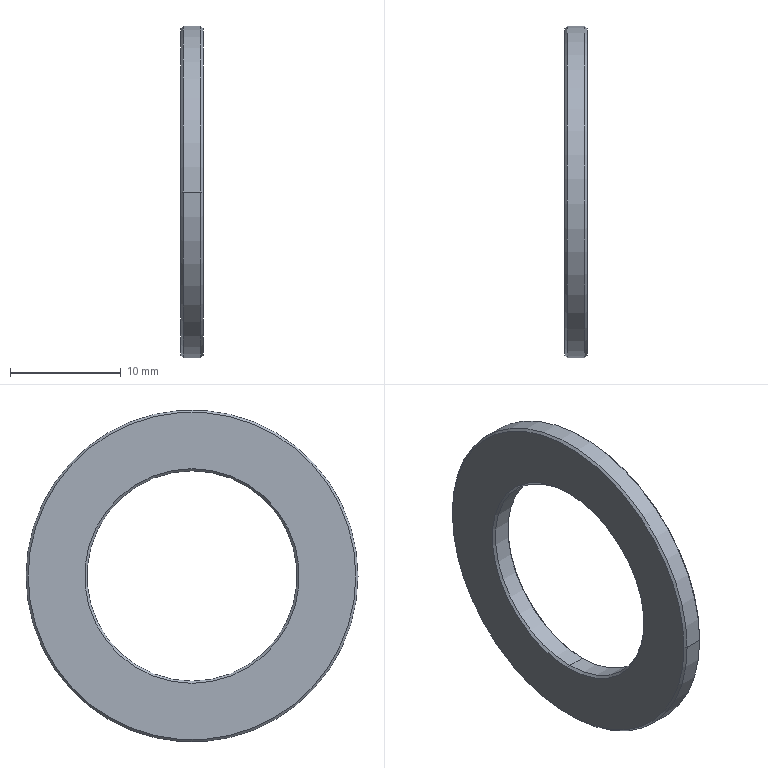Part | STEP file | FWSSS-D30-V19-T2.0 | 1 solid | 14 faces | box 2 x 30 x 30 mm | volume 840.502 mm3 | cone 8 | cylinder 4 | plane 2 | commonest cylinder face diameters 19 x2 30 x2
STEP:
#1=CARTESIAN_POINT('',(0.,0.,0.));
#2=DIRECTION('',(0.,0.,1.));
#3=DIRECTION('',(1.,0.,0.));
#4=AXIS2_PLACEMENT_3D('',#1,#2,#3);
#5=CARTESIAN_POINT('',(0.2,0.,9.5));
#6=VERTEX_POINT('',#5);
#7=CARTESIAN_POINT('',(0.,0.,9.7));
#8=VERTEX_POINT('',#7);
#9=CARTESIAN_POINT('',(0.2,0.,9.5));
#10=DIRECTION('',(-0.7071,0.,0.7071));
#11=VECTOR('',#10,1.);
#12=LINE('',#9,#11);
#13=CARTESIAN_POINT('',(0.2,0.,0.));
#14=DIRECTION('',(-1.,0.,0.));
#15=DIRECTION('',(0.,0.,1.));
#16=AXIS2_PLACEMENT_3D('',#13,#14,#15);
#17=CONICAL_SURFACE('',#16,9.5,0.7854);
#18=CARTESIAN_POINT('',(6.283,0.));
#19=DIRECTION('',(0.,1.));
#20=VECTOR('',#19,1.);
#21=LINE('',#18,#20);
#22=(GEOMETRIC_REPRESENTATION_CONTEXT(2)PARAMETRIC_REPRESENTATION_CONTEXT()REPRESENTATION_CONTEXT('',''));
#23=DEFINITIONAL_REPRESENTATION('',(#21),#22);
#24=PCURVE('',#17,#23);
#25=CARTESIAN_POINT('',(0.2,0.,0.));
#26=DIRECTION('',(-1.,0.,0.));
#27=DIRECTION('',(0.,0.,1.));
#28=AXIS2_PLACEMENT_3D('',#25,#26,#27);
#29=CONICAL_SURFACE('',#28,9.5,0.7854);
#30=CARTESIAN_POINT('',(0.,0.));
#31=DIRECTION('',(0.,1.));
#32=VECTOR('',#31,1.);
#33=LINE('',#30,#32);
#34=(GEOMETRIC_REPRESENTATION_CONTEXT(2)PARAMETRIC_REPRESENTATION_CONTEXT()REPRESENTATION_CONTEXT('',''));
#35=DEFINITIONAL_REPRESENTATION('',(#33),#34);
#36=PCURVE('',#29,#35);
#37=SURFACE_CURVE('',#12,(#24,#36),.PCURVE_S1.);
#38=EDGE_CURVE('',#6,#8,#37,.T.);
#39=ORIENTED_EDGE('',*,*,#38,.T.);
#40=CARTESIAN_POINT('',(0.,0.,-9.7));
#41=VERTEX_POINT('',#40);
#42=CARTESIAN_POINT('',(0.,0.,0.));
#43=DIRECTION('',(1.,0.,0.));
#44=DIRECTION('',(0.,1.,0.));
#45=AXIS2_PLACEMENT_3D('',#42,#43,#44);
#46=CIRCLE('',#45,9.7);
#47=CARTESIAN_POINT('',(7.854,0.2));
#48=DIRECTION('',(-1.,0.));
#49=VECTOR('',#48,1.);
#50=LINE('',#47,#49);
#51=(GEOMETRIC_REPRESENTATION_CONTEXT(2)PARAMETRIC_REPRESENTATION_CONTEXT()REPRESENTATION_CONTEXT('',''));
#52=DEFINITIONAL_REPRESENTATION('',(#50),#51);
#53=PCURVE('',#17,#52);
#54=CARTESIAN_POINT('',(0.,15.,0.));
#55=DIRECTION('',(1.,0.,0.));
#56=DIRECTION('',(0.,1.,0.));
#57=AXIS2_PLACEMENT_3D('',#54,#55,#56);
#58=PLANE('',#57);
#59=CARTESIAN_POINT('',(-15.,0.));
#60=DIRECTION('',(1.,0.));
#61=AXIS2_PLACEMENT_2D('',#59,#60);
#62=CIRCLE('',#61,9.7);
#63=(GEOMETRIC_REPRESENTATION_CONTEXT(2)PARAMETRIC_REPRESENTATION_CONTEXT()REPRESENTATION_CONTEXT('',''));
#64=DEFINITIONAL_REPRESENTATION('',(#62),#63);
#65=PCURVE('',#58,#64);
#66=SURFACE_CURVE('',#46,(#53,#65),.PCURVE_S1.);
#67=EDGE_CURVE('',#8,#41,#66,.T.);
#68=ORIENTED_EDGE('',*,*,#67,.T.);
#69=CARTESIAN_POINT('',(0.2,0.,-9.5));
#70=VERTEX_POINT('',#69);
#71=CARTESIAN_POINT('',(0.2,0.,-9.5));
#72=DIRECTION('',(-0.7071,0.,-0.7071));
#73=VECTOR('',#72,1.);
#74=LINE('',#71,#73);
#75=CARTESIAN_POINT('',(3.142,0.));
#76=DIRECTION('',(0.,1.));
#77=VECTOR('',#76,1.);
#78=LINE('',#75,#77);
#79=(GEOMETRIC_REPRESENTATION_CONTEXT(2)PARAMETRIC_REPRESENTATION_CONTEXT()REPRESENTATION_CONTEXT('',''));
#80=DEFINITIONAL_REPRESENTATION('',(#78),#79);
#81=PCURVE('',#17,#80);
#82=CARTESIAN_POINT('',(3.142,0.));
#83=DIRECTION('',(0.,1.));
#84=VECTOR('',#83,1.);
#85=LINE('',#82,#84);
#86=(GEOMETRIC_REPRESENTATION_CONTEXT(2)PARAMETRIC_REPRESENTATION_CONTEXT()REPRESENTATION_CONTEXT('',''));
#87=DEFINITIONAL_REPRESENTATION('',(#85),#86);
#88=PCURVE('',#29,#87);
#89=SURFACE_CURVE('',#74,(#81,#88),.PCURVE_S1.);
#90=EDGE_CURVE('',#70,#41,#89,.T.);
#91=ORIENTED_EDGE('',*,*,#90,.F.);
#92=CARTESIAN_POINT('',(0.2,0.,0.));
#93=DIRECTION('',(-1.,0.,0.));
#94=DIRECTION('',(0.,0.,-1.));
#95=AXIS2_PLACEMENT_3D('',#92,#93,#94);
#96=CIRCLE('',#95,9.5);
#97=CARTESIAN_POINT('',(3.142,0.));
#98=DIRECTION('',(1.,0.));
#99=VECTOR('',#98,1.);
#100=LINE('',#97,#99);
#101=(GEOMETRIC_REPRESENTATION_CONTEXT(2)PARAMETRIC_REPRESENTATION_CONTEXT()REPRESENTATION_CONTEXT('',''));
#102=DEFINITIONAL_REPRESENTATION('',(#100),#101);
#103=PCURVE('',#17,#102);
#104=CARTESIAN_POINT('',(0.,0.,0.));
#105=DIRECTION('',(1.,0.,0.));
#106=DIRECTION('',(0.,0.,-1.));
#107=AXIS2_PLACEMENT_3D('',#104,#105,#106);
#108=CYLINDRICAL_SURFACE('',#107,9.5);
#109=CARTESIAN_POINT('',(6.283,0.2));
#110=DIRECTION('',(-1.,0.));
#111=VECTOR('',#110,1.);
#112=LINE('',#109,#111);
#113=(GEOMETRIC_REPRESENTATION_CONTEXT(2)PARAMETRIC_REPRESENTATION_CONTEXT()REPRESENTATION_CONTEXT('',''));
#114=DEFINITIONAL_REPRESENTATION('',(#112),#113);
#115=PCURVE('',#108,#114);
#116=SURFACE_CURVE('',#96,(#103,#115),.PCURVE_S1.);
#117=EDGE_CURVE('',#70,#6,#116,.T.);
#118=ORIENTED_EDGE('',*,*,#117,.T.);
#119=EDGE_LOOP('',(#39,#68,#91,#118));
#120=FACE_BOUND('',#119,.F.);
#121=ADVANCED_FACE('',(#120),#17,.F.);
#122=CARTESIAN_POINT('',(1.8,0.,-9.5));
#123=VERTEX_POINT('',#122);
#124=CARTESIAN_POINT('',(2.,0.,-9.7));
#125=VERTEX_POINT('',#124);
#126=CARTESIAN_POINT('',(1.8,0.,-9.5));
#127=DIRECTION('',(0.7071,0.,-0.7071));
#128=VECTOR('',#127,1.);
#129=LINE('',#126,#128);
#130=CARTESIAN_POINT('',(1.8,0.,0.));
#131=DIRECTION('',(1.,0.,0.));
#132=DIRECTION('',(0.,0.,-1.));
#133=AXIS2_PLACEMENT_3D('',#130,#131,#132);
#134=CONICAL_SURFACE('',#133,9.5,0.7854);
#135=CARTESIAN_POINT('',(6.283,0.));
#136=DIRECTION('',(0.,1.));
#137=VECTOR('',#136,1.);
#138=LINE('',#135,#137);
#139=(GEOMETRIC_REPRESENTATION_CONTEXT(2)PARAMETRIC_REPRESENTATION_CONTEXT()REPRESENTATION_CONTEXT('',''));
#140=DEFINITIONAL_REPRESENTATION('',(#138),#139);
#141=PCURVE('',#134,#140);
#142=CARTESIAN_POINT('',(1.8,0.,0.));
#143=DIRECTION('',(1.,0.,0.));
#144=DIRECTION('',(0.,0.,-1.));
#145=AXIS2_PLACEMENT_3D('',#142,#143,#144);
#146=CONICAL_SURFACE('',#145,9.5,0.7854);
#147=CARTESIAN_POINT('',(0.,0.));
#148=DIRECTION('',(0.,1.));
#149=VECTOR('',#148,1.);
#150=LINE('',#147,#149);
#151=(GEOMETRIC_REPRESENTATION_CONTEXT(2)PARAMETRIC_REPRESENTATION_CONTEXT()REPRESENTATION_CONTEXT('',''));
#152=DEFINITIONAL_REPRESENTATION('',(#150),#151);
#153=PCURVE('',#146,#152);
#154=SURFACE_CURVE('',#129,(#141,#153),.PCURVE_S1.);
#155=EDGE_CURVE('',#123,#125,#154,.T.);
#156=ORIENTED_EDGE('',*,*,#155,.T.);
#157=CARTESIAN_POINT('',(2.,0.,9.7));
#158=VERTEX_POINT('',#157);
#159=CARTESIAN_POINT('',(2.,0.,0.));
#160=DIRECTION('',(-1.,0.,0.));
#161=DIRECTION('',(0.,-1.,0.));
#162=AXIS2_PLACEMENT_3D('',#159,#160,#161);
#163=CIRCLE('',#162,9.7);
#164=CARTESIAN_POINT('',(10.996,0.2));
#165=DIRECTION('',(-1.,0.));
#166=VECTOR('',#165,1.);
#167=LINE('',#164,#166);
#168=(GEOMETRIC_REPRESENTATION_CONTEXT(2)PARAMETRIC_REPRESENTATION_CONTEXT()REPRESENTATION_CONTEXT('',''));
#169=DEFINITIONAL_REPRESENTATION('',(#167),#168);
#170=PCURVE('',#134,#169);
#171=CARTESIAN_POINT('',(2.,15.,0.));
#172=DIRECTION('',(-1.,0.,0.));
#173=DIRECTION('',(0.,-1.,0.));
#174=AXIS2_PLACEMENT_3D('',#171,#172,#173);
#175=PLANE('',#174);
#176=CARTESIAN_POINT('',(15.,0.));
#177=DIRECTION('',(1.,0.));
#178=AXIS2_PLACEMENT_2D('',#176,#177);
#179=CIRCLE('',#178,9.7);
#180=(GEOMETRIC_REPRESENTATION_CONTEXT(2)PARAMETRIC_REPRESENTATION_CONTEXT()REPRESENTATION_CONTEXT('',''));
#181=DEFINITIONAL_REPRESENTATION('',(#179),#180);
#182=PCURVE('',#175,#181);
#183=SURFACE_CURVE('',#163,(#170,#182),.PCURVE_S1.);
#184=EDGE_CURVE('',#125,#158,#183,.T.);
#185=ORIENTED_EDGE('',*,*,#184,.T.);
#186=CARTESIAN_POINT('',(1.8,0.,9.5));
#187=VERTEX_POINT('',#186);
#188=CARTESIAN_POINT('',(1.8,0.,9.5));
#189=DIRECTION('',(0.7071,0.,0.7071));
#190=VECTOR('',#189,1.);
#191=LINE('',#188,#190);
#192=CARTESIAN_POINT('',(3.142,0.));
#193=DIRECTION('',(0.,1.));
#194=VECTOR('',#193,1.);
#195=LINE('',#192,#194);
#196=(GEOMETRIC_REPRESENTATION_CONTEXT(2)PARAMETRIC_REPRESENTATION_CONTEXT()REPRESENTATION_CONTEXT('',''));
#197=DEFINITIONAL_REPRESENTATION('',(#195),#196);
#198=PCURVE('',#134,#197);
#199=CARTESIAN_POINT('',(3.142,0.));
#200=DIRECTION('',(0.,1.));
#201=VECTOR('',#200,1.);
#202=LINE('',#199,#201);
#203=(GEOMETRIC_REPRESENTATION_CONTEXT(2)PARAMETRIC_REPRESENTATION_CONTEXT()REPRESENTATION_CONTEXT('',''));
#204=DEFINITIONAL_REPRESENTATION('',(#202),#203);
#205=PCURVE('',#146,#204);
#206=SURFACE_CURVE('',#191,(#198,#205),.PCURVE_S1.);
#207=EDGE_CURVE('',#187,#158,#206,.T.);
#208=ORIENTED_EDGE('',*,*,#207,.F.);
#209=CARTESIAN_POINT('',(1.8,0.,0.));
#210=DIRECTION('',(1.,0.,0.));
#211=DIRECTION('',(0.,0.,1.));
#212=AXIS2_PLACEMENT_3D('',#209,#210,#211);
#213=CIRCLE('',#212,9.5);
#214=CARTESIAN_POINT('',(3.142,0.));
#215=DIRECTION('',(1.,0.));
#216=VECTOR('',#215,1.);
#217=LINE('',#214,#216);
#218=(GEOMETRIC_REPRESENTATION_CONTEXT(2)PARAMETRIC_REPRESENTATION_CONTEXT()REPRESENTATION_CONTEXT('',''));
#219=DEFINITIONAL_REPRESENTATION('',(#217),#218);
#220=PCURVE('',#134,#219);
#221=CARTESIAN_POINT('',(3.142,1.8));
#222=DIRECTION('',(1.,0.));
#223=VECTOR('',#222,1.);
#224=LINE('',#221,#223);
#225=(GEOMETRIC_REPRESENTATION_CONTEXT(2)PARAMETRIC_REPRESENTATION_CONTEXT()REPRESENTATION_CONTEXT('',''));
#226=DEFINITIONAL_REPRESENTATION('',(#224),#225);
#227=PCURVE('',#108,#226);
#228=SURFACE_CURVE('',#213,(#220,#227),.PCURVE_S1.);
#229=EDGE_CURVE('',#187,#123,#228,.T.);
#230=ORIENTED_EDGE('',*,*,#229,.T.);
#231=EDGE_LOOP('',(#156,#185,#208,#230));
#232=FACE_BOUND('',#231,.F.);
#233=ADVANCED_FACE('',(#232),#134,.F.);
#234=CARTESIAN_POINT('',(2.,14.8,0.));
#235=VERTEX_POINT('',#234);
#236=CARTESIAN_POINT('',(2.,-14.8,0.));
#237=VERTEX_POINT('',#236);
#238=CARTESIAN_POINT('',(2.,0.,0.));
#239=DIRECTION('',(1.,0.,0.));
#240=DIRECTION('',(0.,-1.,0.));
#241=AXIS2_PLACEMENT_3D('',#238,#239,#240);
#242=CIRCLE('',#241,14.8);
#243=CARTESIAN_POINT('',(1.8,0.,0.));
#244=DIRECTION('',(-1.,0.,0.));
#245=DIRECTION('',(0.,-1.,0.));
#246=AXIS2_PLACEMENT_3D('',#243,#244,#245);
#247=CONICAL_SURFACE('',#246,15.,0.7854);
#248=CARTESIAN_POINT('',(6.283,-0.2));
#249=DIRECTION('',(-1.,0.));
#250=VECTOR('',#249,1.);
#251=LINE('',#248,#250);
#252=(GEOMETRIC_REPRESENTATION_CONTEXT(2)PARAMETRIC_REPRESENTATION_CONTEXT()REPRESENTATION_CONTEXT('',''));
#253=DEFINITIONAL_REPRESENTATION('',(#251),#252);
#254=PCURVE('',#247,#253);
#255=CARTESIAN_POINT('',(29.8,0.));
#256=CARTESIAN_POINT('',(29.8,-25.634));
#257=CARTESIAN_POINT('',(7.6,-12.817));
#258=CARTESIAN_POINT('',(-14.6,0.));
#259=CARTESIAN_POINT('',(7.6,12.817));
#260=CARTESIAN_POINT('',(29.8,25.634));
#261=CARTESIAN_POINT('',(29.8,0.));
#262=(BOUNDED_CURVE()B_SPLINE_CURVE(2,(#255,#256,#257,#258,#259,#260,#261),.UNSPECIFIED.,.T.,.F.)B_SPLINE_CURVE_WITH_KNOTS((1,2,2,2,2,1),(-2.094,0.,2.094,4.189,6.283,8.378),.UNSPECIFIED.)CURVE()GEOMETRIC_REPRESENTATION_ITEM()RATIONAL_B_SPLINE_CURVE((1.,0.5,1.,0.5,1.,0.5,1.))REPRESENTATION_ITEM(''));
#263=(GEOMETRIC_REPRESENTATION_CONTEXT(2)PARAMETRIC_REPRESENTATION_CONTEXT()REPRESENTATION_CONTEXT('',''));
#264=DEFINITIONAL_REPRESENTATION('',(#262),#263);
#265=PCURVE('',#175,#264);
#266=SURFACE_CURVE('',#242,(#254,#265),.PCURVE_S1.);
#267=EDGE_CURVE('',#235,#237,#266,.T.);
#268=ORIENTED_EDGE('',*,*,#267,.F.);
#269=CARTESIAN_POINT('',(1.8,15.,0.));
#270=VERTEX_POINT('',#269);
#271=CARTESIAN_POINT('',(1.8,15.,0.));
#272=DIRECTION('',(-0.7071,0.7071,0.));
#273=VECTOR('',#272,1.);
#274=LINE('',#271,#273);
#275=CARTESIAN_POINT('',(3.142,0.));
#276=DIRECTION('',(0.,1.));
#277=VECTOR('',#276,1.);
#278=LINE('',#275,#277);
#279=(GEOMETRIC_REPRESENTATION_CONTEXT(2)PARAMETRIC_REPRESENTATION_CONTEXT()REPRESENTATION_CONTEXT('',''));
#280=DEFINITIONAL_REPRESENTATION('',(#278),#279);
#281=PCURVE('',#247,#280);
#282=CARTESIAN_POINT('',(1.8,0.,0.));
#283=DIRECTION('',(-1.,0.,0.));
#284=DIRECTION('',(0.,-1.,0.));
#285=AXIS2_PLACEMENT_3D('',#282,#283,#284);
#286=CONICAL_SURFACE('',#285,15.,0.7854);
#287=CARTESIAN_POINT('',(3.142,0.));
#288=DIRECTION('',(0.,1.));
#289=VECTOR('',#288,1.);
#290=LINE('',#287,#289);
#291=(GEOMETRIC_REPRESENTATION_CONTEXT(2)PARAMETRIC_REPRESENTATION_CONTEXT()REPRESENTATION_CONTEXT('',''));
#292=DEFINITIONAL_REPRESENTATION('',(#290),#291);
#293=PCURVE('',#286,#292);
#294=SURFACE_CURVE('',#274,(#281,#293),.PCURVE_S1.);
#295=EDGE_CURVE('',#235,#270,#294,.T.);
#296=ORIENTED_EDGE('',*,*,#295,.T.);
#297=CARTESIAN_POINT('',(1.8,-15.,0.));
#298=VERTEX_POINT('',#297);
#299=CARTESIAN_POINT('',(1.8,0.,0.));
#300=DIRECTION('',(-1.,0.,0.));
#301=DIRECTION('',(0.,-1.,0.));
#302=AXIS2_PLACEMENT_3D('',#299,#300,#301);
#303=CIRCLE('',#302,15.);
#304=CARTESIAN_POINT('',(0.,0.));
#305=DIRECTION('',(1.,0.));
#306=VECTOR('',#305,1.);
#307=LINE('',#304,#306);
#308=(GEOMETRIC_REPRESENTATION_CONTEXT(2)PARAMETRIC_REPRESENTATION_CONTEXT()REPRESENTATION_CONTEXT('',''));
#309=DEFINITIONAL_REPRESENTATION('',(#307),#308);
#310=PCURVE('',#247,#309);
#311=CARTESIAN_POINT('',(0.,0.,0.));
#312=DIRECTION('',(-1.,0.,0.));
#313=DIRECTION('',(0.,-1.,0.));
#314=AXIS2_PLACEMENT_3D('',#311,#312,#313);
#315=CYLINDRICAL_SURFACE('',#314,15.);
#316=CARTESIAN_POINT('',(0.,-1.8));
#317=DIRECTION('',(1.,0.));
#318=VECTOR('',#317,1.);
#319=LINE('',#316,#318);
#320=(GEOMETRIC_REPRESENTATION_CONTEXT(2)PARAMETRIC_REPRESENTATION_CONTEXT()REPRESENTATION_CONTEXT('',''));
#321=DEFINITIONAL_REPRESENTATION('',(#319),#320);
#322=PCURVE('',#315,#321);
#323=SURFACE_CURVE('',#303,(#310,#322),.PCURVE_S1.);
#324=EDGE_CURVE('',#298,#270,#323,.T.);
#325=ORIENTED_EDGE('',*,*,#324,.F.);
#326=CARTESIAN_POINT('',(1.8,-15.,0.));
#327=DIRECTION('',(-0.7071,-0.7071,0.));
#328=VECTOR('',#327,1.);
#329=LINE('',#326,#328);
#330=CARTESIAN_POINT('',(0.,0.));
#331=DIRECTION('',(0.,1.));
#332=VECTOR('',#331,1.);
#333=LINE('',#330,#332);
#334=(GEOMETRIC_REPRESENTATION_CONTEXT(2)PARAMETRIC_REPRESENTATION_CONTEXT()REPRESENTATION_CONTEXT('',''));
#335=DEFINITIONAL_REPRESENTATION('',(#333),#334);
#336=PCURVE('',#247,#335);
#337=CARTESIAN_POINT('',(6.283,0.));
#338=DIRECTION('',(0.,1.));
#339=VECTOR('',#338,1.);
#340=LINE('',#337,#339);
#341=(GEOMETRIC_REPRESENTATION_CONTEXT(2)PARAMETRIC_REPRESENTATION_CONTEXT()REPRESENTATION_CONTEXT('',''));
#342=DEFINITIONAL_REPRESENTATION('',(#340),#341);
#343=PCURVE('',#286,#342);
#344=SURFACE_CURVE('',#329,(#336,#343),.PCURVE_S1.);
#345=EDGE_CURVE('',#237,#298,#344,.T.);
#346=ORIENTED_EDGE('',*,*,#345,.F.);
#347=EDGE_LOOP('',(#268,#296,#325,#346));
#348=FACE_BOUND('',#347,.T.);
#349=ADVANCED_FACE('',(#348),#247,.T.);
#350=CARTESIAN_POINT('',(0.,-14.8,0.));
#351=VERTEX_POINT('',#350);
#352=CARTESIAN_POINT('',(0.,14.8,0.));
#353=VERTEX_POINT('',#352);
#354=CARTESIAN_POINT('',(0.,0.,0.));
#355=DIRECTION('',(-1.,0.,0.));
#356=DIRECTION('',(0.,1.,0.));
#357=AXIS2_PLACEMENT_3D('',#354,#355,#356);
#358=CIRCLE('',#357,14.8);
#359=CARTESIAN_POINT('',(0.,0.,0.));
#360=DIRECTION('',(1.,0.,0.));
#361=DIRECTION('',(0.,1.,0.));
#362=AXIS2_PLACEMENT_3D('',#359,#360,#361);
#363=CONICAL_SURFACE('',#362,14.8,0.7854);
#364=CARTESIAN_POINT('',(6.283,0.));
#365=DIRECTION('',(-1.,0.));
#366=VECTOR('',#365,1.);
#367=LINE('',#364,#366);
#368=(GEOMETRIC_REPRESENTATION_CONTEXT(2)PARAMETRIC_REPRESENTATION_CONTEXT()REPRESENTATION_CONTEXT('',''));
#369=DEFINITIONAL_REPRESENTATION('',(#367),#368);
#370=PCURVE('',#363,#369);
#371=CARTESIAN_POINT('',(-0.2,0.));
#372=CARTESIAN_POINT('',(-0.2,-25.634));
#373=CARTESIAN_POINT('',(-22.4,-12.817));
#374=CARTESIAN_POINT('',(-44.6,0.));
#375=CARTESIAN_POINT('',(-22.4,12.817));
#376=CARTESIAN_POINT('',(-0.2,25.634));
#377=CARTESIAN_POINT('',(-0.2,0.));
#378=(BOUNDED_CURVE()B_SPLINE_CURVE(2,(#371,#372,#373,#374,#375,#376,#377),.UNSPECIFIED.,.T.,.F.)B_SPLINE_CURVE_WITH_KNOTS((1,2,2,2,2,1),(-2.094,0.,2.094,4.189,6.283,8.378),.UNSPECIFIED.)CURVE()GEOMETRIC_REPRESENTATION_ITEM()RATIONAL_B_SPLINE_CURVE((1.,0.5,1.,0.5,1.,0.5,1.))REPRESENTATION_ITEM(''));
#379=(GEOMETRIC_REPRESENTATION_CONTEXT(2)PARAMETRIC_REPRESENTATION_CONTEXT()REPRESENTATION_CONTEXT('',''));
#380=DEFINITIONAL_REPRESENTATION('',(#378),#379);
#381=PCURVE('',#58,#380);
#382=SURFACE_CURVE('',#358,(#370,#381),.PCURVE_S1.);
#383=EDGE_CURVE('',#351,#353,#382,.T.);
#384=ORIENTED_EDGE('',*,*,#383,.F.);
#385=CARTESIAN_POINT('',(0.2,-15.,0.));
#386=VERTEX_POINT('',#385);
#387=CARTESIAN_POINT('',(0.,-14.8,0.));
#388=DIRECTION('',(0.7071,-0.7071,0.));
#389=VECTOR('',#388,1.);
#390=LINE('',#387,#389);
#391=CARTESIAN_POINT('',(3.142,0.));
#392=DIRECTION('',(0.,1.));
#393=VECTOR('',#392,1.);
#394=LINE('',#391,#393);
#395=(GEOMETRIC_REPRESENTATION_CONTEXT(2)PARAMETRIC_REPRESENTATION_CONTEXT()REPRESENTATION_CONTEXT('',''));
#396=DEFINITIONAL_REPRESENTATION('',(#394),#395);
#397=PCURVE('',#363,#396);
#398=CARTESIAN_POINT('',(0.,0.,0.));
#399=DIRECTION('',(1.,0.,0.));
#400=DIRECTION('',(0.,1.,0.));
#401=AXIS2_PLACEMENT_3D('',#398,#399,#400);
#402=CONICAL_SURFACE('',#401,14.8,0.7854);
#403=CARTESIAN_POINT('',(3.142,0.));
#404=DIRECTION('',(0.,1.));
#405=VECTOR('',#404,1.);
#406=LINE('',#403,#405);
#407=(GEOMETRIC_REPRESENTATION_CONTEXT(2)PARAMETRIC_REPRESENTATION_CONTEXT()REPRESENTATION_CONTEXT('',''));
#408=DEFINITIONAL_REPRESENTATION('',(#406),#407);
#409=PCURVE('',#402,#408);
#410=SURFACE_CURVE('',#390,(#397,#409),.PCURVE_S1.);
#411=EDGE_CURVE('',#351,#386,#410,.T.);
#412=ORIENTED_EDGE('',*,*,#411,.T.);
#413=CARTESIAN_POINT('',(0.2,15.,0.));
#414=VERTEX_POINT('',#413);
#415=CARTESIAN_POINT('',(0.2,0.,0.));
#416=DIRECTION('',(1.,0.,0.));
#417=DIRECTION('',(0.,1.,0.));
#418=AXIS2_PLACEMENT_3D('',#415,#416,#417);
#419=CIRCLE('',#418,15.);
#420=CARTESIAN_POINT('',(0.,0.2));
#421=DIRECTION('',(1.,0.));
#422=VECTOR('',#421,1.);
#423=LINE('',#420,#422);
#424=(GEOMETRIC_REPRESENTATION_CONTEXT(2)PARAMETRIC_REPRESENTATION_CONTEXT()REPRESENTATION_CONTEXT('',''));
#425=DEFINITIONAL_REPRESENTATION('',(#423),#424);
#426=PCURVE('',#363,#425);
#427=CARTESIAN_POINT('',(3.142,-0.2));
#428=DIRECTION('',(-1.,0.));
#429=VECTOR('',#428,1.);
#430=LINE('',#427,#429);
#431=(GEOMETRIC_REPRESENTATION_CONTEXT(2)PARAMETRIC_REPRESENTATION_CONTEXT()REPRESENTATION_CONTEXT('',''));
#432=DEFINITIONAL_REPRESENTATION('',(#430),#431);
#433=PCURVE('',#315,#432);
#434=SURFACE_CURVE('',#419,(#426,#433),.PCURVE_S1.);
#435=EDGE_CURVE('',#414,#386,#434,.T.);
#436=ORIENTED_EDGE('',*,*,#435,.F.);
#437=CARTESIAN_POINT('',(0.,14.8,0.));
#438=DIRECTION('',(0.7071,0.7071,0.));
#439=VECTOR('',#438,1.);
#440=LINE('',#437,#439);
#441=CARTESIAN_POINT('',(0.,0.));
#442=DIRECTION('',(0.,1.));
#443=VECTOR('',#442,1.);
#444=LINE('',#441,#443);
#445=(GEOMETRIC_REPRESENTATION_CONTEXT(2)PARAMETRIC_REPRESENTATION_CONTEXT()REPRESENTATION_CONTEXT('',''));
#446=DEFINITIONAL_REPRESENTATION('',(#444),#445);
#447=PCURVE('',#363,#446);
#448=CARTESIAN_POINT('',(6.283,0.));
#449=DIRECTION('',(0.,1.));
#450=VECTOR('',#449,1.);
#451=LINE('',#448,#450);
#452=(GEOMETRIC_REPRESENTATION_CONTEXT(2)PARAMETRIC_REPRESENTATION_CONTEXT()REPRESENTATION_CONTEXT('',''));
#453=DEFINITIONAL_REPRESENTATION('',(#451),#452);
#454=PCURVE('',#402,#453);
#455=SURFACE_CURVE('',#440,(#447,#454),.PCURVE_S1.);
#456=EDGE_CURVE('',#353,#414,#455,.T.);
#457=ORIENTED_EDGE('',*,*,#456,.F.);
#458=EDGE_LOOP('',(#384,#412,#436,#457));
#459=FACE_BOUND('',#458,.T.);
#460=ADVANCED_FACE('',(#459),#363,.T.);
#461=CARTESIAN_POINT('',(0.,0.,-9.5));
#462=DIRECTION('',(1.,0.,0.));
#463=VECTOR('',#462,1.);
#464=LINE('',#461,#463);
#465=CARTESIAN_POINT('',(6.283,0.));
#466=DIRECTION('',(0.,1.));
#467=VECTOR('',#466,1.);
#468=LINE('',#465,#467);
#469=(GEOMETRIC_REPRESENTATION_CONTEXT(2)PARAMETRIC_REPRESENTATION_CONTEXT()REPRESENTATION_CONTEXT('',''));
#470=DEFINITIONAL_REPRESENTATION('',(#468),#469);
#471=PCURVE('',#108,#470);
#472=CARTESIAN_POINT('',(0.,0.,0.));
#473=DIRECTION('',(1.,0.,0.));
#474=DIRECTION('',(0.,0.,-1.));
#475=AXIS2_PLACEMENT_3D('',#472,#473,#474);
#476=CYLINDRICAL_SURFACE('',#475,9.5);
#477=CARTESIAN_POINT('',(0.,0.));
#478=DIRECTION('',(0.,1.));
#479=VECTOR('',#478,1.);
#480=LINE('',#477,#479);
#481=(GEOMETRIC_REPRESENTATION_CONTEXT(2)PARAMETRIC_REPRESENTATION_CONTEXT()REPRESENTATION_CONTEXT('',''));
#482=DEFINITIONAL_REPRESENTATION('',(#480),#481);
#483=PCURVE('',#476,#482);
#484=SURFACE_CURVE('',#464,(#471,#483),.PCURVE_S1.);
#485=EDGE_CURVE('',#70,#123,#484,.T.);
#486=ORIENTED_EDGE('',*,*,#485,.T.);
#487=ORIENTED_EDGE('',*,*,#229,.F.);
#488=CARTESIAN_POINT('',(0.,0.,9.5));
#489=DIRECTION('',(1.,0.,0.));
#490=VECTOR('',#489,1.);
#491=LINE('',#488,#490);
#492=CARTESIAN_POINT('',(3.142,0.));
#493=DIRECTION('',(0.,1.));
#494=VECTOR('',#493,1.);
#495=LINE('',#492,#494);
#496=(GEOMETRIC_REPRESENTATION_CONTEXT(2)PARAMETRIC_REPRESENTATION_CONTEXT()REPRESENTATION_CONTEXT('',''));
#497=DEFINITIONAL_REPRESENTATION('',(#495),#496);
#498=PCURVE('',#108,#497);
#499=CARTESIAN_POINT('',(3.142,0.));
#500=DIRECTION('',(0.,1.));
#501=VECTOR('',#500,1.);
#502=LINE('',#499,#501);
#503=(GEOMETRIC_REPRESENTATION_CONTEXT(2)PARAMETRIC_REPRESENTATION_CONTEXT()REPRESENTATION_CONTEXT('',''));
#504=DEFINITIONAL_REPRESENTATION('',(#502),#503);
#505=PCURVE('',#476,#504);
#506=SURFACE_CURVE('',#491,(#498,#505),.PCURVE_S1.);
#507=EDGE_CURVE('',#6,#187,#506,.T.);
#508=ORIENTED_EDGE('',*,*,#507,.F.);
#509=ORIENTED_EDGE('',*,*,#117,.F.);
#510=EDGE_LOOP('',(#486,#487,#508,#509));
#511=FACE_BOUND('',#510,.F.);
#512=ADVANCED_FACE('',(#511),#108,.F.);
#513=ORIENTED_EDGE('',*,*,#324,.T.);
#514=CARTESIAN_POINT('',(0.,15.,0.));
#515=DIRECTION('',(-1.,0.,0.));
#516=VECTOR('',#515,1.);
#517=LINE('',#514,#516);
#518=CARTESIAN_POINT('',(3.142,0.));
#519=DIRECTION('',(0.,1.));
#520=VECTOR('',#519,1.);
#521=LINE('',#518,#520);
#522=(GEOMETRIC_REPRESENTATION_CONTEXT(2)PARAMETRIC_REPRESENTATION_CONTEXT()REPRESENTATION_CONTEXT('',''));
#523=DEFINITIONAL_REPRESENTATION('',(#521),#522);
#524=PCURVE('',#315,#523);
#525=CARTESIAN_POINT('',(0.,0.,0.));
#526=DIRECTION('',(-1.,0.,0.));
#527=DIRECTION('',(0.,-1.,0.));
#528=AXIS2_PLACEMENT_3D('',#525,#526,#527);
#529=CYLINDRICAL_SURFACE('',#528,15.);
#530=CARTESIAN_POINT('',(3.142,0.));
#531=DIRECTION('',(0.,1.));
#532=VECTOR('',#531,1.);
#533=LINE('',#530,#532);
#534=(GEOMETRIC_REPRESENTATION_CONTEXT(2)PARAMETRIC_REPRESENTATION_CONTEXT()REPRESENTATION_CONTEXT('',''));
#535=DEFINITIONAL_REPRESENTATION('',(#533),#534);
#536=PCURVE('',#529,#535);
#537=SURFACE_CURVE('',#517,(#524,#536),.PCURVE_S1.);
#538=EDGE_CURVE('',#270,#414,#537,.T.);
#539=ORIENTED_EDGE('',*,*,#538,.T.);
#540=ORIENTED_EDGE('',*,*,#435,.T.);
#541=CARTESIAN_POINT('',(0.,-15.,0.));
#542=DIRECTION('',(-1.,0.,0.));
#543=VECTOR('',#542,1.);
#544=LINE('',#541,#543);
#545=CARTESIAN_POINT('',(0.,0.));
#546=DIRECTION('',(0.,1.));
#547=VECTOR('',#546,1.);
#548=LINE('',#545,#547);
#549=(GEOMETRIC_REPRESENTATION_CONTEXT(2)PARAMETRIC_REPRESENTATION_CONTEXT()REPRESENTATION_CONTEXT('',''));
#550=DEFINITIONAL_REPRESENTATION('',(#548),#549);
#551=PCURVE('',#315,#550);
#552=CARTESIAN_POINT('',(6.283,0.));
#553=DIRECTION('',(0.,1.));
#554=VECTOR('',#553,1.);
#555=LINE('',#552,#554);
#556=(GEOMETRIC_REPRESENTATION_CONTEXT(2)PARAMETRIC_REPRESENTATION_CONTEXT()REPRESENTATION_CONTEXT('',''));
#557=DEFINITIONAL_REPRESENTATION('',(#555),#556);
#558=PCURVE('',#529,#557);
#559=SURFACE_CURVE('',#544,(#551,#558),.PCURVE_S1.);
#560=EDGE_CURVE('',#298,#386,#559,.T.);
#561=ORIENTED_EDGE('',*,*,#560,.F.);
#562=EDGE_LOOP('',(#513,#539,#540,#561));
#563=FACE_BOUND('',#562,.T.);
#564=ADVANCED_FACE('',(#563),#315,.T.);
#565=ORIENTED_EDGE('',*,*,#184,.T.);
#566=CARTESIAN_POINT('',(2.,0.,0.));
#567=DIRECTION('',(-1.,0.,0.));
#568=DIRECTION('',(0.,-1.,0.));
#569=AXIS2_PLACEMENT_3D('',#566,#567,#568);
#570=CIRCLE('',#569,9.7);
#571=CARTESIAN_POINT('',(15.,0.));
#572=DIRECTION('',(1.,0.));
#573=AXIS2_PLACEMENT_2D('',#571,#572);
#574=CIRCLE('',#573,9.7);
#575=(GEOMETRIC_REPRESENTATION_CONTEXT(2)PARAMETRIC_REPRESENTATION_CONTEXT()REPRESENTATION_CONTEXT('',''));
#576=DEFINITIONAL_REPRESENTATION('',(#574),#575);
#577=PCURVE('',#175,#576);
#578=CARTESIAN_POINT('',(4.712,0.2));
#579=DIRECTION('',(-1.,0.));
#580=VECTOR('',#579,1.);
#581=LINE('',#578,#580);
#582=(GEOMETRIC_REPRESENTATION_CONTEXT(2)PARAMETRIC_REPRESENTATION_CONTEXT()REPRESENTATION_CONTEXT('',''));
#583=DEFINITIONAL_REPRESENTATION('',(#581),#582);
#584=PCURVE('',#146,#583);
#585=SURFACE_CURVE('',#570,(#577,#584),.PCURVE_S1.);
#586=EDGE_CURVE('',#158,#125,#585,.T.);
#587=ORIENTED_EDGE('',*,*,#586,.T.);
#588=EDGE_LOOP('',(#565,#587));
#589=FACE_BOUND('',#588,.T.);
#590=CARTESIAN_POINT('',(2.,0.,0.));
#591=DIRECTION('',(1.,0.,0.));
#592=DIRECTION('',(0.,-1.,0.));
#593=AXIS2_PLACEMENT_3D('',#590,#591,#592);
#594=CIRCLE('',#593,14.8);
#595=CARTESIAN_POINT('',(29.8,0.));
#596=CARTESIAN_POINT('',(29.8,-25.634));
#597=CARTESIAN_POINT('',(7.6,-12.817));
#598=CARTESIAN_POINT('',(-14.6,0.));
#599=CARTESIAN_POINT('',(7.6,12.817));
#600=CARTESIAN_POINT('',(29.8,25.634));
#601=CARTESIAN_POINT('',(29.8,0.));
#602=(BOUNDED_CURVE()B_SPLINE_CURVE(2,(#595,#596,#597,#598,#599,#600,#601),.UNSPECIFIED.,.T.,.F.)B_SPLINE_CURVE_WITH_KNOTS((1,2,2,2,2,1),(-2.094,0.,2.094,4.189,6.283,8.378),.UNSPECIFIED.)CURVE()GEOMETRIC_REPRESENTATION_ITEM()RATIONAL_B_SPLINE_CURVE((1.,0.5,1.,0.5,1.,0.5,1.))REPRESENTATION_ITEM(''));
#603=(GEOMETRIC_REPRESENTATION_CONTEXT(2)PARAMETRIC_REPRESENTATION_CONTEXT()REPRESENTATION_CONTEXT('',''));
#604=DEFINITIONAL_REPRESENTATION('',(#602),#603);
#605=PCURVE('',#175,#604);
#606=CARTESIAN_POINT('',(6.283,-0.2));
#607=DIRECTION('',(-1.,0.));
#608=VECTOR('',#607,1.);
#609=LINE('',#606,#608);
#610=(GEOMETRIC_REPRESENTATION_CONTEXT(2)PARAMETRIC_REPRESENTATION_CONTEXT()REPRESENTATION_CONTEXT('',''));
#611=DEFINITIONAL_REPRESENTATION('',(#609),#610);
#612=PCURVE('',#286,#611);
#613=SURFACE_CURVE('',#594,(#605,#612),.PCURVE_S1.);
#614=EDGE_CURVE('',#237,#235,#613,.T.);
#615=ORIENTED_EDGE('',*,*,#614,.T.);
#616=ORIENTED_EDGE('',*,*,#267,.T.);
#617=EDGE_LOOP('',(#615,#616));
#618=FACE_BOUND('',#617,.T.);
#619=ADVANCED_FACE('',(#589,#618),#175,.F.);
#620=ORIENTED_EDGE('',*,*,#67,.T.);
#621=CARTESIAN_POINT('',(0.,0.,0.));
#622=DIRECTION('',(1.,0.,0.));
#623=DIRECTION('',(0.,1.,0.));
#624=AXIS2_PLACEMENT_3D('',#621,#622,#623);
#625=CIRCLE('',#624,9.7);
#626=CARTESIAN_POINT('',(-15.,0.));
#627=DIRECTION('',(1.,0.));
#628=AXIS2_PLACEMENT_2D('',#626,#627);
#629=CIRCLE('',#628,9.7);
#630=(GEOMETRIC_REPRESENTATION_CONTEXT(2)PARAMETRIC_REPRESENTATION_CONTEXT()REPRESENTATION_CONTEXT('',''));
#631=DEFINITIONAL_REPRESENTATION('',(#629),#630);
#632=PCURVE('',#58,#631);
#633=CARTESIAN_POINT('',(7.854,0.2));
#634=DIRECTION('',(-1.,0.));
#635=VECTOR('',#634,1.);
#636=LINE('',#633,#635);
#637=(GEOMETRIC_REPRESENTATION_CONTEXT(2)PARAMETRIC_REPRESENTATION_CONTEXT()REPRESENTATION_CONTEXT('',''));
#638=DEFINITIONAL_REPRESENTATION('',(#636),#637);
#639=PCURVE('',#29,#638);
#640=SURFACE_CURVE('',#625,(#632,#639),.PCURVE_S1.);
#641=EDGE_CURVE('',#41,#8,#640,.T.);
#642=ORIENTED_EDGE('',*,*,#641,.T.);
#643=EDGE_LOOP('',(#620,#642));
#644=FACE_BOUND('',#643,.T.);
#645=CARTESIAN_POINT('',(0.,0.,0.));
#646=DIRECTION('',(-1.,0.,0.));
#647=DIRECTION('',(0.,1.,0.));
#648=AXIS2_PLACEMENT_3D('',#645,#646,#647);
#649=CIRCLE('',#648,14.8);
#650=CARTESIAN_POINT('',(-0.2,0.));
#651=CARTESIAN_POINT('',(-0.2,-25.634));
#652=CARTESIAN_POINT('',(-22.4,-12.817));
#653=CARTESIAN_POINT('',(-44.6,0.));
#654=CARTESIAN_POINT('',(-22.4,12.817));
#655=CARTESIAN_POINT('',(-0.2,25.634));
#656=CARTESIAN_POINT('',(-0.2,0.));
#657=(BOUNDED_CURVE()B_SPLINE_CURVE(2,(#650,#651,#652,#653,#654,#655,#656),.UNSPECIFIED.,.T.,.F.)B_SPLINE_CURVE_WITH_KNOTS((1,2,2,2,2,1),(-2.094,0.,2.094,4.189,6.283,8.378),.UNSPECIFIED.)CURVE()GEOMETRIC_REPRESENTATION_ITEM()RATIONAL_B_SPLINE_CURVE((1.,0.5,1.,0.5,1.,0.5,1.))REPRESENTATION_ITEM(''));
#658=(GEOMETRIC_REPRESENTATION_CONTEXT(2)PARAMETRIC_REPRESENTATION_CONTEXT()REPRESENTATION_CONTEXT('',''));
#659=DEFINITIONAL_REPRESENTATION('',(#657),#658);
#660=PCURVE('',#58,#659);
#661=CARTESIAN_POINT('',(6.283,0.));
#662=DIRECTION('',(-1.,0.));
#663=VECTOR('',#662,1.);
#664=LINE('',#661,#663);
#665=(GEOMETRIC_REPRESENTATION_CONTEXT(2)PARAMETRIC_REPRESENTATION_CONTEXT()REPRESENTATION_CONTEXT('',''));
#666=DEFINITIONAL_REPRESENTATION('',(#664),#665);
#667=PCURVE('',#402,#666);
#668=SURFACE_CURVE('',#649,(#660,#667),.PCURVE_S1.);
#669=EDGE_CURVE('',#353,#351,#668,.T.);
#670=ORIENTED_EDGE('',*,*,#669,.T.);
#671=ORIENTED_EDGE('',*,*,#383,.T.);
#672=EDGE_LOOP('',(#670,#671));
#673=FACE_BOUND('',#672,.T.);
#674=ADVANCED_FACE('',(#644,#673),#58,.F.);
#675=ORIENTED_EDGE('',*,*,#538,.F.);
#676=CARTESIAN_POINT('',(1.8,0.,0.));
#677=DIRECTION('',(-1.,0.,0.));
#678=DIRECTION('',(0.,-1.,0.));
#679=AXIS2_PLACEMENT_3D('',#676,#677,#678);
#680=CIRCLE('',#679,15.);
#681=CARTESIAN_POINT('',(0.,-1.8));
#682=DIRECTION('',(1.,0.));
#683=VECTOR('',#682,1.);
#684=LINE('',#681,#683);
#685=(GEOMETRIC_REPRESENTATION_CONTEXT(2)PARAMETRIC_REPRESENTATION_CONTEXT()REPRESENTATION_CONTEXT('',''));
#686=DEFINITIONAL_REPRESENTATION('',(#684),#685);
#687=PCURVE('',#529,#686);
#688=CARTESIAN_POINT('',(0.,0.));
#689=DIRECTION('',(1.,0.));
#690=VECTOR('',#689,1.);
#691=LINE('',#688,#690);
#692=(GEOMETRIC_REPRESENTATION_CONTEXT(2)PARAMETRIC_REPRESENTATION_CONTEXT()REPRESENTATION_CONTEXT('',''));
#693=DEFINITIONAL_REPRESENTATION('',(#691),#692);
#694=PCURVE('',#286,#693);
#695=SURFACE_CURVE('',#680,(#687,#694),.PCURVE_S1.);
#696=EDGE_CURVE('',#270,#298,#695,.T.);
#697=ORIENTED_EDGE('',*,*,#696,.T.);
#698=ORIENTED_EDGE('',*,*,#560,.T.);
#699=CARTESIAN_POINT('',(0.2,0.,0.));
#700=DIRECTION('',(1.,0.,0.));
#701=DIRECTION('',(0.,1.,0.));
#702=AXIS2_PLACEMENT_3D('',#699,#700,#701);
#703=CIRCLE('',#702,15.);
#704=CARTESIAN_POINT('',(9.425,-0.2));
#705=DIRECTION('',(-1.,0.));
#706=VECTOR('',#705,1.);
#707=LINE('',#704,#706);
#708=(GEOMETRIC_REPRESENTATION_CONTEXT(2)PARAMETRIC_REPRESENTATION_CONTEXT()REPRESENTATION_CONTEXT('',''));
#709=DEFINITIONAL_REPRESENTATION('',(#707),#708);
#710=PCURVE('',#529,#709);
#711=CARTESIAN_POINT('',(0.,0.2));
#712=DIRECTION('',(1.,0.));
#713=VECTOR('',#712,1.);
#714=LINE('',#711,#713);
#715=(GEOMETRIC_REPRESENTATION_CONTEXT(2)PARAMETRIC_REPRESENTATION_CONTEXT()REPRESENTATION_CONTEXT('',''));
#716=DEFINITIONAL_REPRESENTATION('',(#714),#715);
#717=PCURVE('',#402,#716);
#718=SURFACE_CURVE('',#703,(#710,#717),.PCURVE_S1.);
#719=EDGE_CURVE('',#386,#414,#718,.T.);
#720=ORIENTED_EDGE('',*,*,#719,.T.);
#721=EDGE_LOOP('',(#675,#697,#698,#720));
#722=FACE_BOUND('',#721,.T.);
#723=ADVANCED_FACE('',(#722),#529,.T.);
#724=CARTESIAN_POINT('',(1.8,0.,0.));
#725=DIRECTION('',(1.,0.,0.));
#726=DIRECTION('',(0.,0.,1.));
#727=AXIS2_PLACEMENT_3D('',#724,#725,#726);
#728=CIRCLE('',#727,9.5);
#729=CARTESIAN_POINT('',(-3.142,1.8));
#730=DIRECTION('',(1.,0.));
#731=VECTOR('',#730,1.);
#732=LINE('',#729,#731);
#733=(GEOMETRIC_REPRESENTATION_CONTEXT(2)PARAMETRIC_REPRESENTATION_CONTEXT()REPRESENTATION_CONTEXT('',''));
#734=DEFINITIONAL_REPRESENTATION('',(#732),#733);
#735=PCURVE('',#476,#734);
#736=CARTESIAN_POINT('',(-3.142,0.));
#737=DIRECTION('',(1.,0.));
#738=VECTOR('',#737,1.);
#739=LINE('',#736,#738);
#740=(GEOMETRIC_REPRESENTATION_CONTEXT(2)PARAMETRIC_REPRESENTATION_CONTEXT()REPRESENTATION_CONTEXT('',''));
#741=DEFINITIONAL_REPRESENTATION('',(#739),#740);
#742=PCURVE('',#146,#741);
#743=SURFACE_CURVE('',#728,(#735,#742),.PCURVE_S1.);
#744=EDGE_CURVE('',#123,#187,#743,.T.);
#745=ORIENTED_EDGE('',*,*,#744,.F.);
#746=ORIENTED_EDGE('',*,*,#485,.F.);
#747=CARTESIAN_POINT('',(0.2,0.,0.));
#748=DIRECTION('',(-1.,0.,0.));
#749=DIRECTION('',(0.,0.,-1.));
#750=AXIS2_PLACEMENT_3D('',#747,#748,#749);
#751=CIRCLE('',#750,9.5);
#752=CARTESIAN_POINT('',(6.283,0.2));
#753=DIRECTION('',(-1.,0.));
#754=VECTOR('',#753,1.);
#755=LINE('',#752,#754);
#756=(GEOMETRIC_REPRESENTATION_CONTEXT(2)PARAMETRIC_REPRESENTATION_CONTEXT()REPRESENTATION_CONTEXT('',''));
#757=DEFINITIONAL_REPRESENTATION('',(#755),#756);
#758=PCURVE('',#476,#757);
#759=CARTESIAN_POINT('',(-3.142,0.));
#760=DIRECTION('',(1.,0.));
#761=VECTOR('',#760,1.);
#762=LINE('',#759,#761);
#763=(GEOMETRIC_REPRESENTATION_CONTEXT(2)PARAMETRIC_REPRESENTATION_CONTEXT()REPRESENTATION_CONTEXT('',''));
#764=DEFINITIONAL_REPRESENTATION('',(#762),#763);
#765=PCURVE('',#29,#764);
#766=SURFACE_CURVE('',#751,(#758,#765),.PCURVE_S1.);
#767=EDGE_CURVE('',#6,#70,#766,.T.);
#768=ORIENTED_EDGE('',*,*,#767,.F.);
#769=ORIENTED_EDGE('',*,*,#507,.T.);
#770=EDGE_LOOP('',(#745,#746,#768,#769));
#771=FACE_BOUND('',#770,.F.);
#772=ADVANCED_FACE('',(#771),#476,.F.);
#773=ORIENTED_EDGE('',*,*,#411,.F.);
#774=ORIENTED_EDGE('',*,*,#669,.F.);
#775=ORIENTED_EDGE('',*,*,#456,.T.);
#776=ORIENTED_EDGE('',*,*,#719,.F.);
#777=EDGE_LOOP('',(#773,#774,#775,#776));
#778=FACE_BOUND('',#777,.T.);
#779=ADVANCED_FACE('',(#778),#402,.T.);
#780=ORIENTED_EDGE('',*,*,#295,.F.);
#781=ORIENTED_EDGE('',*,*,#614,.F.);
#782=ORIENTED_EDGE('',*,*,#345,.T.);
#783=ORIENTED_EDGE('',*,*,#696,.F.);
#784=EDGE_LOOP('',(#780,#781,#782,#783));
#785=FACE_BOUND('',#784,.T.);
#786=ADVANCED_FACE('',(#785),#286,.T.);
#787=ORIENTED_EDGE('',*,*,#586,.T.);
#788=ORIENTED_EDGE('',*,*,#155,.F.);
#789=ORIENTED_EDGE('',*,*,#744,.T.);
#790=ORIENTED_EDGE('',*,*,#207,.T.);
#791=EDGE_LOOP('',(#787,#788,#789,#790));
#792=FACE_BOUND('',#791,.F.);
#793=ADVANCED_FACE('',(#792),#146,.F.);
#794=ORIENTED_EDGE('',*,*,#641,.T.);
#795=ORIENTED_EDGE('',*,*,#38,.F.);
#796=ORIENTED_EDGE('',*,*,#767,.T.);
#797=ORIENTED_EDGE('',*,*,#90,.T.);
#798=EDGE_LOOP('',(#794,#795,#796,#797));
#799=FACE_BOUND('',#798,.F.);
#800=ADVANCED_FACE('',(#799),#29,.F.);
#801=CLOSED_SHELL('',(#121,#233,#349,#460,#512,#564,#619,#674,#723,#772,#779,#786,#793,#800));
#802=MANIFOLD_SOLID_BREP('',#801);
#803=(LENGTH_UNIT()NAMED_UNIT(*)SI_UNIT(.MILLI.,.METRE.));
#804=UNCERTAINTY_MEASURE_WITH_UNIT(LENGTH_MEASURE(0.0000001),#803,'','');
#805=(NAMED_UNIT(*)PLANE_ANGLE_UNIT()SI_UNIT($,.RADIAN.));
#806=(NAMED_UNIT(*)SI_UNIT($,.STERADIAN.)SOLID_ANGLE_UNIT());
#807=(GEOMETRIC_REPRESENTATION_CONTEXT(3)GLOBAL_UNCERTAINTY_ASSIGNED_CONTEXT((#804))GLOBAL_UNIT_ASSIGNED_CONTEXT((#803,#805,#806))REPRESENTATION_CONTEXT('',''));
#808=ADVANCED_BREP_SHAPE_REPRESENTATION('',(#4,#802),#807);